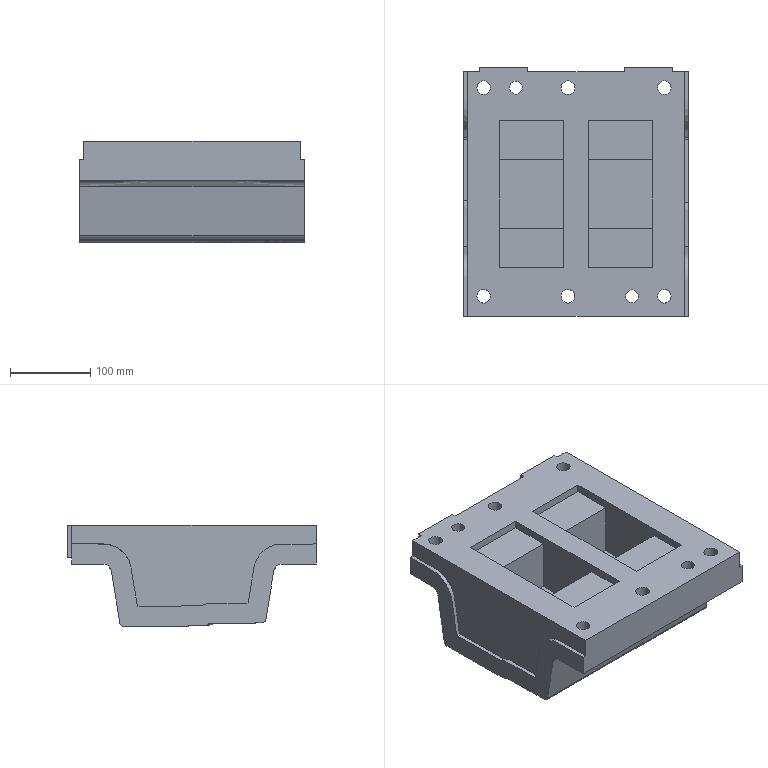Part | NX | features solid 2 | 1 solid | 97 faces | box 280.327 x 310 x 126.004 mm | volume 6770468 mm3 | plane 53 | spline 26 | cylinder 18 | commonest cylinder face diameters 17 x6 26 x6 10 x2 12 x2 16 x2